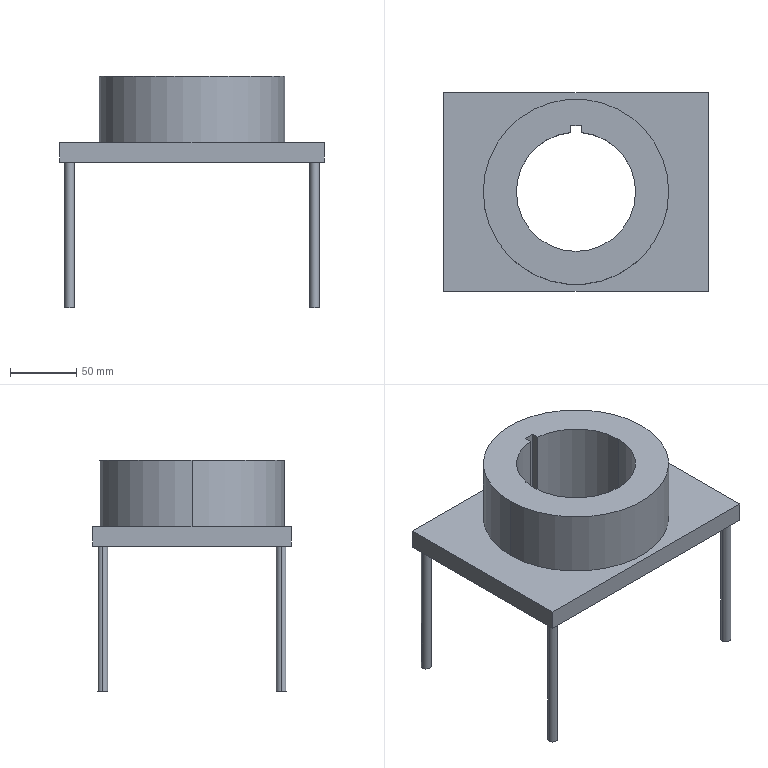Part | SolidWorks | features ICE 4, Cut 1, Extrusion 1 | 2 solids | 30 faces | box 200 x 150 x 175 mm | volume 822892 mm3 | cylinder 15 | plane 15 | commonest cylinder face diameters 7.5 x8 140 x4 90 x3
STEP:
#1=CARTESIAN_POINT('',(70.,0.,-15.));
#2=VERTEX_POINT('',#1);
#3=CARTESIAN_POINT('',(-70.,0.,-15.));
#4=VERTEX_POINT('',#3);
#5=CARTESIAN_POINT('',(0.,0.,-15.));
#6=DIRECTION('',(0.,0.,-1.));
#7=DIRECTION('',(1.,0.,0.));
#8=AXIS2_PLACEMENT_3D('',#5,#6,#7);
#9=CIRCLE('',#8,70.);
#10=EDGE_CURVE('',#2,#4,#9,.T.);
#11=ORIENTED_EDGE('',*,*,#10,.T.);
#12=CARTESIAN_POINT('',(-70.,0.,0.));
#13=VERTEX_POINT('',#12);
#14=CARTESIAN_POINT('',(-70.,0.,-70.));
#15=DIRECTION('',(0.,0.,1.));
#16=VECTOR('',#15,1000.);
#17=LINE('',#14,#16);
#18=EDGE_CURVE('',#4,#13,#17,.T.);
#19=ORIENTED_EDGE('',*,*,#18,.T.);
#20=CARTESIAN_POINT('',(70.,0.,0.));
#21=VERTEX_POINT('',#20);
#22=CARTESIAN_POINT('',(0.,0.,0.));
#23=DIRECTION('',(0.,0.,-1.));
#24=DIRECTION('',(1.,0.,0.));
#25=AXIS2_PLACEMENT_3D('',#22,#23,#24);
#26=CIRCLE('',#25,70.);
#27=EDGE_CURVE('',#21,#13,#26,.T.);
#28=ORIENTED_EDGE('',*,*,#27,.F.);
#29=CARTESIAN_POINT('',(70.,0.,-70.));
#30=DIRECTION('',(0.,0.,1.));
#31=VECTOR('',#30,1000.);
#32=LINE('',#29,#31);
#33=EDGE_CURVE('',#2,#21,#32,.T.);
#34=ORIENTED_EDGE('',*,*,#33,.F.);
#35=EDGE_LOOP('',(#11,#19,#28,#34));
#36=FACE_OUTER_BOUND('',#35,.T.);
#37=CARTESIAN_POINT('',(0.,0.,-70.));
#38=DIRECTION('',(0.,0.,1.));
#39=DIRECTION('',(1.,0.,0.));
#40=AXIS2_PLACEMENT_3D('',#37,#38,#39);
#41=CYLINDRICAL_SURFACE('',#40,70.);
#42=ADVANCED_FACE('',(#36),#41,.F.);
#43=CARTESIAN_POINT('',(88.75,-67.5,-125.));
#44=VERTEX_POINT('',#43);
#45=CARTESIAN_POINT('',(96.25,-67.5,-125.));
#46=VERTEX_POINT('',#45);
#47=CARTESIAN_POINT('',(92.5,-67.5,-125.));
#48=DIRECTION('',(0.,0.,-1.));
#49=DIRECTION('',(1.,0.,0.));
#50=AXIS2_PLACEMENT_3D('',#47,#48,#49);
#51=CIRCLE('',#50,3.75);
#52=EDGE_CURVE('',#44,#46,#51,.T.);
#53=ORIENTED_EDGE('',*,*,#52,.F.);
#54=CARTESIAN_POINT('',(88.75,-67.5,-15.));
#55=VERTEX_POINT('',#54);
#56=CARTESIAN_POINT('',(88.75,-67.5,-125.));
#57=DIRECTION('',(0.,0.,1.));
#58=VECTOR('',#57,1000.);
#59=LINE('',#56,#58);
#60=EDGE_CURVE('',#44,#55,#59,.T.);
#61=ORIENTED_EDGE('',*,*,#60,.T.);
#62=CARTESIAN_POINT('',(96.25,-67.5,-15.));
#63=VERTEX_POINT('',#62);
#64=CARTESIAN_POINT('',(92.5,-67.5,-15.));
#65=DIRECTION('',(0.,0.,-1.));
#66=DIRECTION('',(1.,0.,0.));
#67=AXIS2_PLACEMENT_3D('',#64,#65,#66);
#68=CIRCLE('',#67,3.75);
#69=EDGE_CURVE('',#55,#63,#68,.T.);
#70=ORIENTED_EDGE('',*,*,#69,.T.);
#71=CARTESIAN_POINT('',(96.25,-67.5,-125.));
#72=DIRECTION('',(0.,0.,1.));
#73=VECTOR('',#72,1000.);
#74=LINE('',#71,#73);
#75=EDGE_CURVE('',#46,#63,#74,.T.);
#76=ORIENTED_EDGE('',*,*,#75,.F.);
#77=EDGE_LOOP('',(#53,#61,#70,#76));
#78=FACE_OUTER_BOUND('',#77,.T.);
#79=CARTESIAN_POINT('',(92.5,-67.5,-125.));
#80=DIRECTION('',(0.,0.,1.));
#81=DIRECTION('',(1.,0.,0.));
#82=AXIS2_PLACEMENT_3D('',#79,#80,#81);
#83=CYLINDRICAL_SURFACE('',#82,3.75);
#84=ADVANCED_FACE('',(#78),#83,.T.);
#85=CARTESIAN_POINT('',(-96.25,-67.5,-125.));
#86=VERTEX_POINT('',#85);
#87=CARTESIAN_POINT('',(-88.75,-67.5,-125.));
#88=VERTEX_POINT('',#87);
#89=CARTESIAN_POINT('',(-92.5,-67.5,-125.));
#90=DIRECTION('',(0.,0.,-1.));
#91=DIRECTION('',(-1.,0.,0.));
#92=AXIS2_PLACEMENT_3D('',#89,#90,#91);
#93=CIRCLE('',#92,3.75);
#94=EDGE_CURVE('',#86,#88,#93,.T.);
#95=ORIENTED_EDGE('',*,*,#94,.F.);
#96=CARTESIAN_POINT('',(-96.25,-67.5,-15.));
#97=VERTEX_POINT('',#96);
#98=CARTESIAN_POINT('',(-96.25,-67.5,-125.));
#99=DIRECTION('',(0.,0.,1.));
#100=VECTOR('',#99,1000.);
#101=LINE('',#98,#100);
#102=EDGE_CURVE('',#86,#97,#101,.T.);
#103=ORIENTED_EDGE('',*,*,#102,.T.);
#104=CARTESIAN_POINT('',(-88.75,-67.5,-15.));
#105=VERTEX_POINT('',#104);
#106=CARTESIAN_POINT('',(-92.5,-67.5,-15.));
#107=DIRECTION('',(0.,0.,-1.));
#108=DIRECTION('',(1.,0.,0.));
#109=AXIS2_PLACEMENT_3D('',#106,#107,#108);
#110=CIRCLE('',#109,3.75);
#111=EDGE_CURVE('',#97,#105,#110,.T.);
#112=ORIENTED_EDGE('',*,*,#111,.T.);
#113=CARTESIAN_POINT('',(-88.75,-67.5,-125.));
#114=DIRECTION('',(0.,0.,1.));
#115=VECTOR('',#114,1000.);
#116=LINE('',#113,#115);
#117=EDGE_CURVE('',#88,#105,#116,.T.);
#118=ORIENTED_EDGE('',*,*,#117,.F.);
#119=EDGE_LOOP('',(#95,#103,#112,#118));
#120=FACE_OUTER_BOUND('',#119,.T.);
#121=CARTESIAN_POINT('',(-92.5,-67.5,-125.));
#122=DIRECTION('',(0.,0.,1.));
#123=DIRECTION('',(1.,0.,0.));
#124=AXIS2_PLACEMENT_3D('',#121,#122,#123);
#125=CYLINDRICAL_SURFACE('',#124,3.75);
#126=ADVANCED_FACE('',(#120),#125,.T.);
#127=CARTESIAN_POINT('',(-96.25,67.5,-125.));
#128=VERTEX_POINT('',#127);
#129=CARTESIAN_POINT('',(-88.75,67.5,-125.));
#130=VERTEX_POINT('',#129);
#131=CARTESIAN_POINT('',(-92.5,67.5,-125.));
#132=DIRECTION('',(0.,0.,-1.));
#133=DIRECTION('',(1.,0.,0.));
#134=AXIS2_PLACEMENT_3D('',#131,#132,#133);
#135=CIRCLE('',#134,3.75);
#136=EDGE_CURVE('',#128,#130,#135,.T.);
#137=ORIENTED_EDGE('',*,*,#136,.F.);
#138=CARTESIAN_POINT('',(-96.25,67.5,-15.));
#139=VERTEX_POINT('',#138);
#140=CARTESIAN_POINT('',(-96.25,67.5,-125.));
#141=DIRECTION('',(0.,0.,1.));
#142=VECTOR('',#141,1000.);
#143=LINE('',#140,#142);
#144=EDGE_CURVE('',#128,#139,#143,.T.);
#145=ORIENTED_EDGE('',*,*,#144,.T.);
#146=CARTESIAN_POINT('',(-88.75,67.5,-15.));
#147=VERTEX_POINT('',#146);
#148=CARTESIAN_POINT('',(-92.5,67.5,-15.));
#149=DIRECTION('',(0.,0.,-1.));
#150=DIRECTION('',(1.,0.,0.));
#151=AXIS2_PLACEMENT_3D('',#148,#149,#150);
#152=CIRCLE('',#151,3.75);
#153=EDGE_CURVE('',#139,#147,#152,.T.);
#154=ORIENTED_EDGE('',*,*,#153,.T.);
#155=CARTESIAN_POINT('',(-88.75,67.5,-125.));
#156=DIRECTION('',(0.,0.,1.));
#157=VECTOR('',#156,1000.);
#158=LINE('',#155,#157);
#159=EDGE_CURVE('',#130,#147,#158,.T.);
#160=ORIENTED_EDGE('',*,*,#159,.F.);
#161=EDGE_LOOP('',(#137,#145,#154,#160));
#162=FACE_OUTER_BOUND('',#161,.T.);
#163=CARTESIAN_POINT('',(-92.5,67.5,-125.));
#164=DIRECTION('',(0.,0.,1.));
#165=DIRECTION('',(1.,0.,0.));
#166=AXIS2_PLACEMENT_3D('',#163,#164,#165);
#167=CYLINDRICAL_SURFACE('',#166,3.75);
#168=ADVANCED_FACE('',(#162),#167,.T.);
#169=CARTESIAN_POINT('',(88.75,67.5,-125.));
#170=VERTEX_POINT('',#169);
#171=CARTESIAN_POINT('',(96.25,67.5,-125.));
#172=VERTEX_POINT('',#171);
#173=CARTESIAN_POINT('',(92.5,67.5,-125.));
#174=DIRECTION('',(0.,0.,-1.));
#175=DIRECTION('',(-1.,0.,0.));
#176=AXIS2_PLACEMENT_3D('',#173,#174,#175);
#177=CIRCLE('',#176,3.75);
#178=EDGE_CURVE('',#170,#172,#177,.T.);
#179=ORIENTED_EDGE('',*,*,#178,.F.);
#180=CARTESIAN_POINT('',(88.75,67.5,-15.));
#181=VERTEX_POINT('',#180);
#182=CARTESIAN_POINT('',(88.75,67.5,-125.));
#183=DIRECTION('',(0.,0.,1.));
#184=VECTOR('',#183,1000.);
#185=LINE('',#182,#184);
#186=EDGE_CURVE('',#170,#181,#185,.T.);
#187=ORIENTED_EDGE('',*,*,#186,.T.);
#188=CARTESIAN_POINT('',(96.25,67.5,-15.));
#189=VERTEX_POINT('',#188);
#190=CARTESIAN_POINT('',(92.5,67.5,-15.));
#191=DIRECTION('',(0.,0.,-1.));
#192=DIRECTION('',(1.,0.,0.));
#193=AXIS2_PLACEMENT_3D('',#190,#191,#192);
#194=CIRCLE('',#193,3.75);
#195=EDGE_CURVE('',#181,#189,#194,.T.);
#196=ORIENTED_EDGE('',*,*,#195,.T.);
#197=CARTESIAN_POINT('',(96.25,67.5,-125.));
#198=DIRECTION('',(0.,0.,1.));
#199=VECTOR('',#198,1000.);
#200=LINE('',#197,#199);
#201=EDGE_CURVE('',#172,#189,#200,.T.);
#202=ORIENTED_EDGE('',*,*,#201,.F.);
#203=EDGE_LOOP('',(#179,#187,#196,#202));
#204=FACE_OUTER_BOUND('',#203,.T.);
#205=CARTESIAN_POINT('',(92.5,67.5,-125.));
#206=DIRECTION('',(0.,0.,1.));
#207=DIRECTION('',(1.,0.,0.));
#208=AXIS2_PLACEMENT_3D('',#205,#206,#207);
#209=CYLINDRICAL_SURFACE('',#208,3.75);
#210=ADVANCED_FACE('',(#204),#209,.T.);
#211=CARTESIAN_POINT('',(-100.,-75.,0.));
#212=VERTEX_POINT('',#211);
#213=CARTESIAN_POINT('',(-100.,75.,0.));
#214=VERTEX_POINT('',#213);
#215=CARTESIAN_POINT('',(-100.,-75.,0.));
#216=DIRECTION('',(0.,1.,0.));
#217=VECTOR('',#216,1000.);
#218=LINE('',#215,#217);
#219=EDGE_CURVE('',#212,#214,#218,.T.);
#220=ORIENTED_EDGE('',*,*,#219,.T.);
#221=CARTESIAN_POINT('',(-100.,75.,-15.));
#222=VERTEX_POINT('',#221);
#223=CARTESIAN_POINT('',(-100.,75.,-15.));
#224=DIRECTION('',(0.,0.,1.));
#225=VECTOR('',#224,1000.);
#226=LINE('',#223,#225);
#227=EDGE_CURVE('',#222,#214,#226,.T.);
#228=ORIENTED_EDGE('',*,*,#227,.F.);
#229=CARTESIAN_POINT('',(-100.,-75.,-15.));
#230=VERTEX_POINT('',#229);
#231=CARTESIAN_POINT('',(-100.,-75.,-15.));
#232=DIRECTION('',(0.,1.,0.));
#233=VECTOR('',#232,1000.);
#234=LINE('',#231,#233);
#235=EDGE_CURVE('',#230,#222,#234,.T.);
#236=ORIENTED_EDGE('',*,*,#235,.F.);
#237=CARTESIAN_POINT('',(-100.,-75.,-15.));
#238=DIRECTION('',(0.,0.,1.));
#239=VECTOR('',#238,1000.);
#240=LINE('',#237,#239);
#241=EDGE_CURVE('',#230,#212,#240,.T.);
#242=ORIENTED_EDGE('',*,*,#241,.T.);
#243=EDGE_LOOP('',(#220,#228,#236,#242));
#244=FACE_OUTER_BOUND('',#243,.T.);
#245=CARTESIAN_POINT('',(-100.,-75.,-15.));
#246=DIRECTION('',(1.,0.,0.));
#247=DIRECTION('',(0.,0.,-1.));
#248=AXIS2_PLACEMENT_3D('',#245,#246,#247);
#249=PLANE('',#248);
#250=ADVANCED_FACE('',(#244),#249,.F.);
#251=CARTESIAN_POINT('',(100.,75.,0.));
#252=VERTEX_POINT('',#251);
#253=CARTESIAN_POINT('',(100.,75.,0.));
#254=DIRECTION('',(1.,0.,0.));
#255=VECTOR('',#254,1000.);
#256=LINE('',#253,#255);
#257=EDGE_CURVE('',#214,#252,#256,.T.);
#258=ORIENTED_EDGE('',*,*,#257,.T.);
#259=CARTESIAN_POINT('',(100.,75.,-15.));
#260=VERTEX_POINT('',#259);
#261=CARTESIAN_POINT('',(100.,75.,-15.));
#262=DIRECTION('',(0.,0.,1.));
#263=VECTOR('',#262,1000.);
#264=LINE('',#261,#263);
#265=EDGE_CURVE('',#260,#252,#264,.T.);
#266=ORIENTED_EDGE('',*,*,#265,.F.);
#267=CARTESIAN_POINT('',(100.,75.,-15.));
#268=DIRECTION('',(1.,0.,0.));
#269=VECTOR('',#268,1000.);
#270=LINE('',#267,#269);
#271=EDGE_CURVE('',#222,#260,#270,.T.);
#272=ORIENTED_EDGE('',*,*,#271,.F.);
#273=ORIENTED_EDGE('',*,*,#227,.T.);
#274=EDGE_LOOP('',(#258,#266,#272,#273));
#275=FACE_OUTER_BOUND('',#274,.T.);
#276=CARTESIAN_POINT('',(100.,75.,-15.));
#277=DIRECTION('',(0.,-1.,0.));
#278=DIRECTION('',(0.,0.,-1.));
#279=AXIS2_PLACEMENT_3D('',#276,#277,#278);
#280=PLANE('',#279);
#281=ADVANCED_FACE('',(#275),#280,.F.);
#282=CARTESIAN_POINT('',(100.,-75.,0.));
#283=VERTEX_POINT('',#282);
#284=CARTESIAN_POINT('',(100.,-75.,0.));
#285=DIRECTION('',(0.,-1.,0.));
#286=VECTOR('',#285,1000.);
#287=LINE('',#284,#286);
#288=EDGE_CURVE('',#252,#283,#287,.T.);
#289=ORIENTED_EDGE('',*,*,#288,.T.);
#290=CARTESIAN_POINT('',(100.,-75.,-15.));
#291=VERTEX_POINT('',#290);
#292=CARTESIAN_POINT('',(100.,-75.,-15.));
#293=DIRECTION('',(0.,0.,1.));
#294=VECTOR('',#293,1000.);
#295=LINE('',#292,#294);
#296=EDGE_CURVE('',#291,#283,#295,.T.);
#297=ORIENTED_EDGE('',*,*,#296,.F.);
#298=CARTESIAN_POINT('',(100.,-75.,-15.));
#299=DIRECTION('',(0.,-1.,0.));
#300=VECTOR('',#299,1000.);
#301=LINE('',#298,#300);
#302=EDGE_CURVE('',#260,#291,#301,.T.);
#303=ORIENTED_EDGE('',*,*,#302,.F.);
#304=ORIENTED_EDGE('',*,*,#265,.T.);
#305=EDGE_LOOP('',(#289,#297,#303,#304));
#306=FACE_OUTER_BOUND('',#305,.T.);
#307=CARTESIAN_POINT('',(100.,-75.,-15.));
#308=DIRECTION('',(-1.,0.,0.));
#309=DIRECTION('',(0.,0.,1.));
#310=AXIS2_PLACEMENT_3D('',#307,#308,#309);
#311=PLANE('',#310);
#312=ADVANCED_FACE('',(#306),#311,.F.);
#313=CARTESIAN_POINT('',(100.,-75.,0.));
#314=DIRECTION('',(-1.,0.,0.));
#315=VECTOR('',#314,1000.);
#316=LINE('',#313,#315);
#317=EDGE_CURVE('',#283,#212,#316,.T.);
#318=ORIENTED_EDGE('',*,*,#317,.T.);
#319=ORIENTED_EDGE('',*,*,#241,.F.);
#320=CARTESIAN_POINT('',(100.,-75.,-15.));
#321=DIRECTION('',(-1.,0.,0.));
#322=VECTOR('',#321,1000.);
#323=LINE('',#320,#322);
#324=EDGE_CURVE('',#291,#230,#323,.T.);
#325=ORIENTED_EDGE('',*,*,#324,.F.);
#326=ORIENTED_EDGE('',*,*,#296,.T.);
#327=EDGE_LOOP('',(#318,#319,#325,#326));
#328=FACE_OUTER_BOUND('',#327,.T.);
#329=CARTESIAN_POINT('',(100.,-75.,-15.));
#330=DIRECTION('',(0.,1.,0.));
#331=DIRECTION('',(0.,0.,1.));
#332=AXIS2_PLACEMENT_3D('',#329,#330,#331);
#333=PLANE('',#332);
#334=ADVANCED_FACE('',(#328),#333,.F.);
#335=ORIENTED_EDGE('',*,*,#10,.F.);
#336=CARTESIAN_POINT('',(0.,0.,-15.));
#337=DIRECTION('',(0.,0.,-1.));
#338=DIRECTION('',(1.,0.,0.));
#339=AXIS2_PLACEMENT_3D('',#336,#337,#338);
#340=CIRCLE('',#339,70.);
#341=EDGE_CURVE('',#4,#2,#340,.T.);
#342=ORIENTED_EDGE('',*,*,#341,.F.);
#343=EDGE_LOOP('',(#335,#342));
#344=FACE_BOUND('',#343,.T.);
#345=CARTESIAN_POINT('',(92.5,-67.5,-15.));
#346=DIRECTION('',(0.,0.,-1.));
#347=DIRECTION('',(1.,0.,0.));
#348=AXIS2_PLACEMENT_3D('',#345,#346,#347);
#349=CIRCLE('',#348,3.75);
#350=EDGE_CURVE('',#63,#55,#349,.T.);
#351=ORIENTED_EDGE('',*,*,#350,.F.);
#352=ORIENTED_EDGE('',*,*,#69,.F.);
#353=EDGE_LOOP('',(#351,#352));
#354=FACE_BOUND('',#353,.T.);
#355=CARTESIAN_POINT('',(-92.5,-67.5,-15.));
#356=DIRECTION('',(0.,0.,-1.));
#357=DIRECTION('',(1.,0.,0.));
#358=AXIS2_PLACEMENT_3D('',#355,#356,#357);
#359=CIRCLE('',#358,3.75);
#360=EDGE_CURVE('',#105,#97,#359,.T.);
#361=ORIENTED_EDGE('',*,*,#360,.F.);
#362=ORIENTED_EDGE('',*,*,#111,.F.);
#363=EDGE_LOOP('',(#361,#362));
#364=FACE_BOUND('',#363,.T.);
#365=CARTESIAN_POINT('',(-92.5,67.5,-15.));
#366=DIRECTION('',(0.,0.,-1.));
#367=DIRECTION('',(1.,0.,0.));
#368=AXIS2_PLACEMENT_3D('',#365,#366,#367);
#369=CIRCLE('',#368,3.75);
#370=EDGE_CURVE('',#147,#139,#369,.T.);
#371=ORIENTED_EDGE('',*,*,#370,.F.);
#372=ORIENTED_EDGE('',*,*,#153,.F.);
#373=EDGE_LOOP('',(#371,#372));
#374=FACE_BOUND('',#373,.T.);
#375=CARTESIAN_POINT('',(92.5,67.5,-15.));
#376=DIRECTION('',(0.,0.,-1.));
#377=DIRECTION('',(1.,0.,0.));
#378=AXIS2_PLACEMENT_3D('',#375,#376,#377);
#379=CIRCLE('',#378,3.75);
#380=EDGE_CURVE('',#189,#181,#379,.T.);
#381=ORIENTED_EDGE('',*,*,#380,.F.);
#382=ORIENTED_EDGE('',*,*,#195,.F.);
#383=EDGE_LOOP('',(#381,#382));
#384=FACE_BOUND('',#383,.T.);
#385=ORIENTED_EDGE('',*,*,#235,.T.);
#386=ORIENTED_EDGE('',*,*,#271,.T.);
#387=ORIENTED_EDGE('',*,*,#302,.T.);
#388=ORIENTED_EDGE('',*,*,#324,.T.);
#389=EDGE_LOOP('',(#385,#386,#387,#388));
#390=FACE_OUTER_BOUND('',#389,.T.);
#391=CARTESIAN_POINT('',(0.,0.,-15.));
#392=DIRECTION('',(0.,0.,1.));
#393=DIRECTION('',(1.,0.,0.));
#394=AXIS2_PLACEMENT_3D('',#391,#392,#393);
#395=PLANE('',#394);
#396=ADVANCED_FACE('',(#344,#354,#364,#374,#384,#390),#395,.F.);
#397=ORIENTED_EDGE('',*,*,#27,.T.);
#398=CARTESIAN_POINT('',(0.,0.,0.));
#399=DIRECTION('',(0.,0.,-1.));
#400=DIRECTION('',(1.,0.,0.));
#401=AXIS2_PLACEMENT_3D('',#398,#399,#400);
#402=CIRCLE('',#401,70.);
#403=EDGE_CURVE('',#13,#21,#402,.T.);
#404=ORIENTED_EDGE('',*,*,#403,.T.);
#405=EDGE_LOOP('',(#397,#404));
#406=FACE_BOUND('',#405,.T.);
#407=ORIENTED_EDGE('',*,*,#219,.F.);
#408=ORIENTED_EDGE('',*,*,#317,.F.);
#409=ORIENTED_EDGE('',*,*,#288,.F.);
#410=ORIENTED_EDGE('',*,*,#257,.F.);
#411=EDGE_LOOP('',(#407,#408,#409,#410));
#412=FACE_OUTER_BOUND('',#411,.T.);
#413=CARTESIAN_POINT('',(0.,0.,0.));
#414=DIRECTION('',(0.,0.,1.));
#415=DIRECTION('',(1.,0.,0.));
#416=AXIS2_PLACEMENT_3D('',#413,#414,#415);
#417=PLANE('',#416);
#418=ADVANCED_FACE('',(#406,#412),#417,.T.);
#419=ORIENTED_EDGE('',*,*,#186,.F.);
#420=CARTESIAN_POINT('',(92.5,67.5,-125.));
#421=DIRECTION('',(0.,0.,-1.));
#422=DIRECTION('',(-1.,0.,0.));
#423=AXIS2_PLACEMENT_3D('',#420,#421,#422);
#424=CIRCLE('',#423,3.75);
#425=EDGE_CURVE('',#172,#170,#424,.T.);
#426=ORIENTED_EDGE('',*,*,#425,.F.);
#427=ORIENTED_EDGE('',*,*,#201,.T.);
#428=ORIENTED_EDGE('',*,*,#380,.T.);
#429=EDGE_LOOP('',(#419,#426,#427,#428));
#430=FACE_OUTER_BOUND('',#429,.T.);
#431=CARTESIAN_POINT('',(92.5,67.5,-125.));
#432=DIRECTION('',(0.,0.,1.));
#433=DIRECTION('',(1.,0.,0.));
#434=AXIS2_PLACEMENT_3D('',#431,#432,#433);
#435=CYLINDRICAL_SURFACE('',#434,3.75);
#436=ADVANCED_FACE('',(#430),#435,.T.);
#437=ORIENTED_EDGE('',*,*,#425,.T.);
#438=ORIENTED_EDGE('',*,*,#178,.T.);
#439=EDGE_LOOP('',(#437,#438));
#440=FACE_OUTER_BOUND('',#439,.T.);
#441=CARTESIAN_POINT('',(92.5,67.5,-125.));
#442=DIRECTION('',(0.,0.,-1.));
#443=DIRECTION('',(-1.,0.,0.));
#444=AXIS2_PLACEMENT_3D('',#441,#442,#443);
#445=PLANE('',#444);
#446=ADVANCED_FACE('',(#440),#445,.T.);
#447=ORIENTED_EDGE('',*,*,#144,.F.);
#448=CARTESIAN_POINT('',(-92.5,67.5,-125.));
#449=DIRECTION('',(0.,0.,-1.));
#450=DIRECTION('',(1.,0.,0.));
#451=AXIS2_PLACEMENT_3D('',#448,#449,#450);
#452=CIRCLE('',#451,3.75);
#453=EDGE_CURVE('',#130,#128,#452,.T.);
#454=ORIENTED_EDGE('',*,*,#453,.F.);
#455=ORIENTED_EDGE('',*,*,#159,.T.);
#456=ORIENTED_EDGE('',*,*,#370,.T.);
#457=EDGE_LOOP('',(#447,#454,#455,#456));
#458=FACE_OUTER_BOUND('',#457,.T.);
#459=CARTESIAN_POINT('',(-92.5,67.5,-125.));
#460=DIRECTION('',(0.,0.,1.));
#461=DIRECTION('',(1.,0.,0.));
#462=AXIS2_PLACEMENT_3D('',#459,#460,#461);
#463=CYLINDRICAL_SURFACE('',#462,3.75);
#464=ADVANCED_FACE('',(#458),#463,.T.);
#465=ORIENTED_EDGE('',*,*,#453,.T.);
#466=ORIENTED_EDGE('',*,*,#136,.T.);
#467=EDGE_LOOP('',(#465,#466));
#468=FACE_OUTER_BOUND('',#467,.T.);
#469=CARTESIAN_POINT('',(-92.5,67.5,-125.));
#470=DIRECTION('',(0.,0.,1.));
#471=DIRECTION('',(1.,0.,0.));
#472=AXIS2_PLACEMENT_3D('',#469,#470,#471);
#473=PLANE('',#472);
#474=ADVANCED_FACE('',(#468),#473,.F.);
#475=ORIENTED_EDGE('',*,*,#102,.F.);
#476=CARTESIAN_POINT('',(-92.5,-67.5,-125.));
#477=DIRECTION('',(0.,0.,-1.));
#478=DIRECTION('',(-1.,0.,0.));
#479=AXIS2_PLACEMENT_3D('',#476,#477,#478);
#480=CIRCLE('',#479,3.75);
#481=EDGE_CURVE('',#88,#86,#480,.T.);
#482=ORIENTED_EDGE('',*,*,#481,.F.);
#483=ORIENTED_EDGE('',*,*,#117,.T.);
#484=ORIENTED_EDGE('',*,*,#360,.T.);
#485=EDGE_LOOP('',(#475,#482,#483,#484));
#486=FACE_OUTER_BOUND('',#485,.T.);
#487=CARTESIAN_POINT('',(-92.5,-67.5,-125.));
#488=DIRECTION('',(0.,0.,1.));
#489=DIRECTION('',(1.,0.,0.));
#490=AXIS2_PLACEMENT_3D('',#487,#488,#489);
#491=CYLINDRICAL_SURFACE('',#490,3.75);
#492=ADVANCED_FACE('',(#486),#491,.T.);
#493=ORIENTED_EDGE('',*,*,#481,.T.);
#494=ORIENTED_EDGE('',*,*,#94,.T.);
#495=EDGE_LOOP('',(#493,#494));
#496=FACE_OUTER_BOUND('',#495,.T.);
#497=CARTESIAN_POINT('',(-92.5,-67.5,-125.));
#498=DIRECTION('',(0.,0.,-1.));
#499=DIRECTION('',(-1.,0.,0.));
#500=AXIS2_PLACEMENT_3D('',#497,#498,#499);
#501=PLANE('',#500);
#502=ADVANCED_FACE('',(#496),#501,.T.);
#503=ORIENTED_EDGE('',*,*,#60,.F.);
#504=CARTESIAN_POINT('',(92.5,-67.5,-125.));
#505=DIRECTION('',(0.,0.,-1.));
#506=DIRECTION('',(1.,0.,0.));
#507=AXIS2_PLACEMENT_3D('',#504,#505,#506);
#508=CIRCLE('',#507,3.75);
#509=EDGE_CURVE('',#46,#44,#508,.T.);
#510=ORIENTED_EDGE('',*,*,#509,.F.);
#511=ORIENTED_EDGE('',*,*,#75,.T.);
#512=ORIENTED_EDGE('',*,*,#350,.T.);
#513=EDGE_LOOP('',(#503,#510,#511,#512));
#514=FACE_OUTER_BOUND('',#513,.T.);
#515=CARTESIAN_POINT('',(92.5,-67.5,-125.));
#516=DIRECTION('',(0.,0.,1.));
#517=DIRECTION('',(1.,0.,0.));
#518=AXIS2_PLACEMENT_3D('',#515,#516,#517);
#519=CYLINDRICAL_SURFACE('',#518,3.75);
#520=ADVANCED_FACE('',(#514),#519,.T.);
#521=ORIENTED_EDGE('',*,*,#509,.T.);
#522=ORIENTED_EDGE('',*,*,#52,.T.);
#523=EDGE_LOOP('',(#521,#522));
#524=FACE_OUTER_BOUND('',#523,.T.);
#525=CARTESIAN_POINT('',(92.5,-67.5,-125.));
#526=DIRECTION('',(0.,0.,1.));
#527=DIRECTION('',(1.,0.,0.));
#528=AXIS2_PLACEMENT_3D('',#525,#526,#527);
#529=PLANE('',#528);
#530=ADVANCED_FACE('',(#524),#529,.F.);
#531=ORIENTED_EDGE('',*,*,#18,.F.);
#532=ORIENTED_EDGE('',*,*,#341,.T.);
#533=ORIENTED_EDGE('',*,*,#33,.T.);
#534=ORIENTED_EDGE('',*,*,#403,.F.);
#535=EDGE_LOOP('',(#531,#532,#533,#534));
#536=FACE_OUTER_BOUND('',#535,.T.);
#537=CARTESIAN_POINT('',(0.,0.,-70.));
#538=DIRECTION('',(0.,0.,1.));
#539=DIRECTION('',(1.,0.,0.));
#540=AXIS2_PLACEMENT_3D('',#537,#538,#539);
#541=CYLINDRICAL_SURFACE('',#540,70.);
#542=ADVANCED_FACE('',(#536),#541,.F.);
#543=CLOSED_SHELL('',(#42,#84,#126,#168,#210,#250,#281,#312,#334,#396,#418,#436,#446,#464,#474,#492,#502,#520,#530,#542));
#544=MANIFOLD_SOLID_BREP('',#543);
#545=CARTESIAN_POINT('',(70.,0.,50.));
#546=VERTEX_POINT('',#545);
#547=CARTESIAN_POINT('',(-70.,0.,50.));
#548=VERTEX_POINT('',#547);
#549=CARTESIAN_POINT('',(0.,0.,50.));
#550=DIRECTION('',(0.,0.,1.));
#551=DIRECTION('',(1.,0.,0.));
#552=AXIS2_PLACEMENT_3D('',#549,#550,#551);
#553=CIRCLE('',#552,70.);
#554=EDGE_CURVE('',#546,#548,#553,.T.);
#555=ORIENTED_EDGE('',*,*,#554,.F.);
#556=CARTESIAN_POINT('',(70.,0.,-15.));
#557=VERTEX_POINT('',#556);
#558=CARTESIAN_POINT('',(70.,0.,50.));
#559=DIRECTION('',(0.,0.,-1.));
#560=VECTOR('',#559,1000.);
#561=LINE('',#558,#560);
#562=EDGE_CURVE('',#546,#557,#561,.T.);
#563=ORIENTED_EDGE('',*,*,#562,.T.);
#564=CARTESIAN_POINT('',(-70.,0.,-15.));
#565=VERTEX_POINT('',#564);
#566=CARTESIAN_POINT('',(0.,0.,-15.));
#567=DIRECTION('',(0.,0.,-1.));
#568=DIRECTION('',(-1.,0.,0.));
#569=AXIS2_PLACEMENT_3D('',#566,#567,#568);
#570=CIRCLE('',#569,70.);
#571=EDGE_CURVE('',#565,#557,#570,.T.);
#572=ORIENTED_EDGE('',*,*,#571,.F.);
#573=CARTESIAN_POINT('',(-70.,0.,50.));
#574=DIRECTION('',(0.,0.,-1.));
#575=VECTOR('',#574,1000.);
#576=LINE('',#573,#575);
#577=EDGE_CURVE('',#548,#565,#576,.T.);
#578=ORIENTED_EDGE('',*,*,#577,.F.);
#579=EDGE_LOOP('',(#555,#563,#572,#578));
#580=FACE_OUTER_BOUND('',#579,.T.);
#581=CARTESIAN_POINT('',(0.,0.,50.));
#582=DIRECTION('',(0.,0.,-1.));
#583=DIRECTION('',(-1.,0.,0.));
#584=AXIS2_PLACEMENT_3D('',#581,#582,#583);
#585=CYLINDRICAL_SURFACE('',#584,70.);
#586=ADVANCED_FACE('',(#580),#585,.T.);
#587=CARTESIAN_POINT('',(-45.,0.,50.));
#588=VERTEX_POINT('',#587);
#589=CARTESIAN_POINT('',(45.,0.,50.));
#590=VERTEX_POINT('',#589);
#591=CARTESIAN_POINT('',(0.,0.,50.));
#592=DIRECTION('',(0.,0.,1.));
#593=DIRECTION('',(1.,0.,0.));
#594=AXIS2_PLACEMENT_3D('',#591,#592,#593);
#595=CIRCLE('',#594,45.);
#596=EDGE_CURVE('',#588,#590,#595,.T.);
#597=ORIENTED_EDGE('',*,*,#596,.T.);
#598=CARTESIAN_POINT('',(45.,0.,-15.));
#599=VERTEX_POINT('',#598);
#600=CARTESIAN_POINT('',(45.,0.,50.));
#601=DIRECTION('',(0.,0.,-1.));
#602=VECTOR('',#601,1000.);
#603=LINE('',#600,#602);
#604=EDGE_CURVE('',#590,#599,#603,.T.);
#605=ORIENTED_EDGE('',*,*,#604,.T.);
#606=CARTESIAN_POINT('',(-45.,0.,-15.));
#607=VERTEX_POINT('',#606);
#608=CARTESIAN_POINT('',(0.,0.,-15.));
#609=DIRECTION('',(0.,0.,-1.));
#610=DIRECTION('',(-1.,0.,0.));
#611=AXIS2_PLACEMENT_3D('',#608,#609,#610);
#612=CIRCLE('',#611,45.);
#613=EDGE_CURVE('',#599,#607,#612,.T.);
#614=ORIENTED_EDGE('',*,*,#613,.T.);
#615=CARTESIAN_POINT('',(-45.,0.,50.));
#616=DIRECTION('',(0.,0.,-1.));
#617=VECTOR('',#616,1000.);
#618=LINE('',#615,#617);
#619=EDGE_CURVE('',#588,#607,#618,.T.);
#620=ORIENTED_EDGE('',*,*,#619,.F.);
#621=EDGE_LOOP('',(#597,#605,#614,#620));
#622=FACE_OUTER_BOUND('',#621,.T.);
#623=CARTESIAN_POINT('',(0.,0.,50.));
#624=DIRECTION('',(0.,0.,-1.));
#625=DIRECTION('',(-1.,0.,0.));
#626=AXIS2_PLACEMENT_3D('',#623,#624,#625);
#627=CYLINDRICAL_SURFACE('',#626,45.);
#628=ADVANCED_FACE('',(#622),#627,.F.);
#629=CARTESIAN_POINT('',(-4.,44.822,50.));
#630=VERTEX_POINT('',#629);
#631=CARTESIAN_POINT('',(0.,0.,50.));
#632=DIRECTION('',(0.,0.,1.));
#633=DIRECTION('',(1.,0.,0.));
#634=AXIS2_PLACEMENT_3D('',#631,#632,#633);
#635=CIRCLE('',#634,45.);
#636=EDGE_CURVE('',#630,#588,#635,.T.);
#637=ORIENTED_EDGE('',*,*,#636,.T.);
#638=ORIENTED_EDGE('',*,*,#619,.T.);
#639=CARTESIAN_POINT('',(-4.,44.822,-15.));
#640=VERTEX_POINT('',#639);
#641=CARTESIAN_POINT('',(0.,0.,-15.));
#642=DIRECTION('',(0.,0.,-1.));
#643=DIRECTION('',(-1.,0.,0.));
#644=AXIS2_PLACEMENT_3D('',#641,#642,#643);
#645=CIRCLE('',#644,45.);
#646=EDGE_CURVE('',#607,#640,#645,.T.);
#647=ORIENTED_EDGE('',*,*,#646,.T.);
#648=CARTESIAN_POINT('',(-4.,44.822,50.));
#649=DIRECTION('',(0.,0.,-1.));
#650=VECTOR('',#649,1000.);
#651=LINE('',#648,#650);
#652=EDGE_CURVE('',#630,#640,#651,.T.);
#653=ORIENTED_EDGE('',*,*,#652,.F.);
#654=EDGE_LOOP('',(#637,#638,#647,#653));
#655=FACE_OUTER_BOUND('',#654,.T.);
#656=CARTESIAN_POINT('',(0.,0.,50.));
#657=DIRECTION('',(0.,0.,-1.));
#658=DIRECTION('',(-1.,0.,0.));
#659=AXIS2_PLACEMENT_3D('',#656,#657,#658);
#660=CYLINDRICAL_SURFACE('',#659,45.);
#661=ADVANCED_FACE('',(#655),#660,.F.);
#662=ORIENTED_EDGE('',*,*,#652,.T.);
#663=CARTESIAN_POINT('',(-4.,50.18,-15.));
#664=VERTEX_POINT('',#663);
#665=CARTESIAN_POINT('',(-4.,44.822,-15.));
#666=DIRECTION('',(0.,1.,0.));
#667=VECTOR('',#666,1000.);
#668=LINE('',#665,#667);
#669=EDGE_CURVE('',#640,#664,#668,.T.);
#670=ORIENTED_EDGE('',*,*,#669,.T.);
#671=CARTESIAN_POINT('',(-4.,50.18,50.));
#672=VERTEX_POINT('',#671);
#673=CARTESIAN_POINT('',(-4.,50.18,-10.63));
#674=DIRECTION('',(0.,0.,1.));
#675=VECTOR('',#674,1000.);
#676=LINE('',#673,#675);
#677=EDGE_CURVE('',#664,#672,#676,.T.);
#678=ORIENTED_EDGE('',*,*,#677,.T.);
#679=CARTESIAN_POINT('',(-4.,50.18,50.));
#680=DIRECTION('',(0.,-1.,0.));
#681=VECTOR('',#680,1000.);
#682=LINE('',#679,#681);
#683=EDGE_CURVE('',#672,#630,#682,.T.);
#684=ORIENTED_EDGE('',*,*,#683,.T.);
#685=EDGE_LOOP('',(#662,#670,#678,#684));
#686=FACE_OUTER_BOUND('',#685,.T.);
#687=CARTESIAN_POINT('',(-4.,50.18,-10.63));
#688=DIRECTION('',(-1.,0.,0.));
#689=DIRECTION('',(0.,-1.,0.));
#690=AXIS2_PLACEMENT_3D('',#687,#688,#689);
#691=PLANE('',#690);
#692=ADVANCED_FACE('',(#686),#691,.F.);
#693=ORIENTED_EDGE('',*,*,#677,.F.);
#694=CARTESIAN_POINT('',(4.,50.18,-15.));
#695=VERTEX_POINT('',#694);
#696=CARTESIAN_POINT('',(-4.,50.18,-15.));
#697=DIRECTION('',(1.,0.,0.));
#698=VECTOR('',#697,1000.);
#699=LINE('',#696,#698);
#700=EDGE_CURVE('',#664,#695,#699,.T.);
#701=ORIENTED_EDGE('',*,*,#700,.T.);
#702=CARTESIAN_POINT('',(4.,50.18,50.));
#703=VERTEX_POINT('',#702);
#704=CARTESIAN_POINT('',(4.,50.18,-10.63));
#705=DIRECTION('',(0.,0.,1.));
#706=VECTOR('',#705,1000.);
#707=LINE('',#704,#706);
#708=EDGE_CURVE('',#695,#703,#707,.T.);
#709=ORIENTED_EDGE('',*,*,#708,.T.);
#710=CARTESIAN_POINT('',(-4.,50.18,50.));
#711=DIRECTION('',(-1.,0.,0.));
#712=VECTOR('',#711,1000.);
#713=LINE('',#710,#712);
#714=EDGE_CURVE('',#703,#672,#713,.T.);
#715=ORIENTED_EDGE('',*,*,#714,.T.);
#716=EDGE_LOOP('',(#693,#701,#709,#715));
#717=FACE_OUTER_BOUND('',#716,.T.);
#718=CARTESIAN_POINT('',(-4.,50.18,-10.63));
#719=DIRECTION('',(0.,1.,0.));
#720=DIRECTION('',(0.,0.,1.));
#721=AXIS2_PLACEMENT_3D('',#718,#719,#720);
#722=PLANE('',#721);
#723=ADVANCED_FACE('',(#717),#722,.F.);
#724=CARTESIAN_POINT('',(4.,44.822,-15.));
#725=VERTEX_POINT('',#724);
#726=CARTESIAN_POINT('',(4.,44.822,50.));
#727=VERTEX_POINT('',#726);
#728=CARTESIAN_POINT('',(4.,44.822,50.));
#729=DIRECTION('',(0.,0.,1.));
#730=VECTOR('',#729,1000.);
#731=LINE('',#728,#730);
#732=EDGE_CURVE('',#725,#727,#731,.T.);
#733=ORIENTED_EDGE('',*,*,#732,.T.);
#734=CARTESIAN_POINT('',(4.,50.18,50.));
#735=DIRECTION('',(0.,1.,0.));
#736=VECTOR('',#735,1000.);
#737=LINE('',#734,#736);
#738=EDGE_CURVE('',#727,#703,#737,.T.);
#739=ORIENTED_EDGE('',*,*,#738,.T.);
#740=ORIENTED_EDGE('',*,*,#708,.F.);
#741=CARTESIAN_POINT('',(4.,50.18,-15.));
#742=DIRECTION('',(0.,-1.,0.));
#743=VECTOR('',#742,1000.);
#744=LINE('',#741,#743);
#745=EDGE_CURVE('',#695,#725,#744,.T.);
#746=ORIENTED_EDGE('',*,*,#745,.T.);
#747=EDGE_LOOP('',(#733,#739,#740,#746));
#748=FACE_OUTER_BOUND('',#747,.T.);
#749=CARTESIAN_POINT('',(4.,50.18,-10.63));
#750=DIRECTION('',(1.,0.,0.));
#751=DIRECTION('',(0.,1.,0.));
#752=AXIS2_PLACEMENT_3D('',#749,#750,#751);
#753=PLANE('',#752);
#754=ADVANCED_FACE('',(#748),#753,.F.);
#755=ORIENTED_EDGE('',*,*,#604,.F.);
#756=CARTESIAN_POINT('',(0.,0.,50.));
#757=DIRECTION('',(0.,0.,1.));
#758=DIRECTION('',(1.,0.,0.));
#759=AXIS2_PLACEMENT_3D('',#756,#757,#758);
#760=CIRCLE('',#759,45.);
#761=EDGE_CURVE('',#590,#727,#760,.T.);
#762=ORIENTED_EDGE('',*,*,#761,.T.);
#763=ORIENTED_EDGE('',*,*,#732,.F.);
#764=CARTESIAN_POINT('',(0.,0.,-15.));
#765=DIRECTION('',(0.,0.,-1.));
#766=DIRECTION('',(-1.,0.,0.));
#767=AXIS2_PLACEMENT_3D('',#764,#765,#766);
#768=CIRCLE('',#767,45.);
#769=EDGE_CURVE('',#725,#599,#768,.T.);
#770=ORIENTED_EDGE('',*,*,#769,.T.);
#771=EDGE_LOOP('',(#755,#762,#763,#770));
#772=FACE_OUTER_BOUND('',#771,.T.);
#773=CARTESIAN_POINT('',(0.,0.,50.));
#774=DIRECTION('',(0.,0.,-1.));
#775=DIRECTION('',(-1.,0.,0.));
#776=AXIS2_PLACEMENT_3D('',#773,#774,#775);
#777=CYLINDRICAL_SURFACE('',#776,45.);
#778=ADVANCED_FACE('',(#772),#777,.F.);
#779=ORIENTED_EDGE('',*,*,#683,.F.);
#780=ORIENTED_EDGE('',*,*,#714,.F.);
#781=ORIENTED_EDGE('',*,*,#738,.F.);
#782=ORIENTED_EDGE('',*,*,#761,.F.);
#783=ORIENTED_EDGE('',*,*,#596,.F.);
#784=ORIENTED_EDGE('',*,*,#636,.F.);
#785=EDGE_LOOP('',(#779,#780,#781,#782,#783,#784));
#786=FACE_BOUND('',#785,.T.);
#787=CARTESIAN_POINT('',(0.,0.,50.));
#788=DIRECTION('',(0.,0.,1.));
#789=DIRECTION('',(1.,0.,0.));
#790=AXIS2_PLACEMENT_3D('',#787,#788,#789);
#791=CIRCLE('',#790,70.);
#792=EDGE_CURVE('',#548,#546,#791,.T.);
#793=ORIENTED_EDGE('',*,*,#792,.T.);
#794=ORIENTED_EDGE('',*,*,#554,.T.);
#795=EDGE_LOOP('',(#793,#794));
#796=FACE_OUTER_BOUND('',#795,.T.);
#797=CARTESIAN_POINT('',(0.,0.,50.));
#798=DIRECTION('',(0.,0.,1.));
#799=DIRECTION('',(1.,0.,0.));
#800=AXIS2_PLACEMENT_3D('',#797,#798,#799);
#801=PLANE('',#800);
#802=ADVANCED_FACE('',(#786,#796),#801,.T.);
#803=ORIENTED_EDGE('',*,*,#562,.F.);
#804=ORIENTED_EDGE('',*,*,#792,.F.);
#805=ORIENTED_EDGE('',*,*,#577,.T.);
#806=CARTESIAN_POINT('',(0.,0.,-15.));
#807=DIRECTION('',(0.,0.,-1.));
#808=DIRECTION('',(-1.,0.,0.));
#809=AXIS2_PLACEMENT_3D('',#806,#807,#808);
#810=CIRCLE('',#809,70.);
#811=EDGE_CURVE('',#557,#565,#810,.T.);
#812=ORIENTED_EDGE('',*,*,#811,.F.);
#813=EDGE_LOOP('',(#803,#804,#805,#812));
#814=FACE_OUTER_BOUND('',#813,.T.);
#815=CARTESIAN_POINT('',(0.,0.,50.));
#816=DIRECTION('',(0.,0.,-1.));
#817=DIRECTION('',(-1.,0.,0.));
#818=AXIS2_PLACEMENT_3D('',#815,#816,#817);
#819=CYLINDRICAL_SURFACE('',#818,70.);
#820=ADVANCED_FACE('',(#814),#819,.T.);
#821=ORIENTED_EDGE('',*,*,#571,.T.);
#822=ORIENTED_EDGE('',*,*,#811,.T.);
#823=EDGE_LOOP('',(#821,#822));
#824=FACE_OUTER_BOUND('',#823,.T.);
#825=ORIENTED_EDGE('',*,*,#669,.F.);
#826=ORIENTED_EDGE('',*,*,#646,.F.);
#827=ORIENTED_EDGE('',*,*,#613,.F.);
#828=ORIENTED_EDGE('',*,*,#769,.F.);
#829=ORIENTED_EDGE('',*,*,#745,.F.);
#830=ORIENTED_EDGE('',*,*,#700,.F.);
#831=EDGE_LOOP('',(#825,#826,#827,#828,#829,#830));
#832=FACE_BOUND('',#831,.T.);
#833=CARTESIAN_POINT('',(0.,0.,-15.));
#834=DIRECTION('',(0.,0.,-1.));
#835=DIRECTION('',(-1.,0.,0.));
#836=AXIS2_PLACEMENT_3D('',#833,#834,#835);
#837=PLANE('',#836);
#838=ADVANCED_FACE('',(#824,#832),#837,.T.);
#839=CLOSED_SHELL('',(#586,#628,#661,#692,#723,#754,#778,#802,#820,#838));
#840=MANIFOLD_SOLID_BREP('',#839);
#841=CARTESIAN_POINT('',(0.,0.,0.));
#842=DIRECTION('',(0.,0.,1.));
#843=DIRECTION('',(1.,0.,0.));
#844=AXIS2_PLACEMENT_3D('',#841,#842,#843);
#845=(LENGTH_UNIT()NAMED_UNIT(*)SI_UNIT(.MILLI.,.METRE.));
#846=UNCERTAINTY_MEASURE_WITH_UNIT(LENGTH_MEASURE(0.00001),#845,'','');
#847=(NAMED_UNIT(*)PLANE_ANGLE_UNIT()SI_UNIT($,.RADIAN.));
#848=(NAMED_UNIT(*)SI_UNIT($,.STERADIAN.)SOLID_ANGLE_UNIT());
#849=(GEOMETRIC_REPRESENTATION_CONTEXT(3)GLOBAL_UNCERTAINTY_ASSIGNED_CONTEXT((#846))GLOBAL_UNIT_ASSIGNED_CONTEXT((#845,#847,#848))REPRESENTATION_CONTEXT('',''));
#850=ADVANCED_BREP_SHAPE_REPRESENTATION('',(#544,#840,#844),#849);